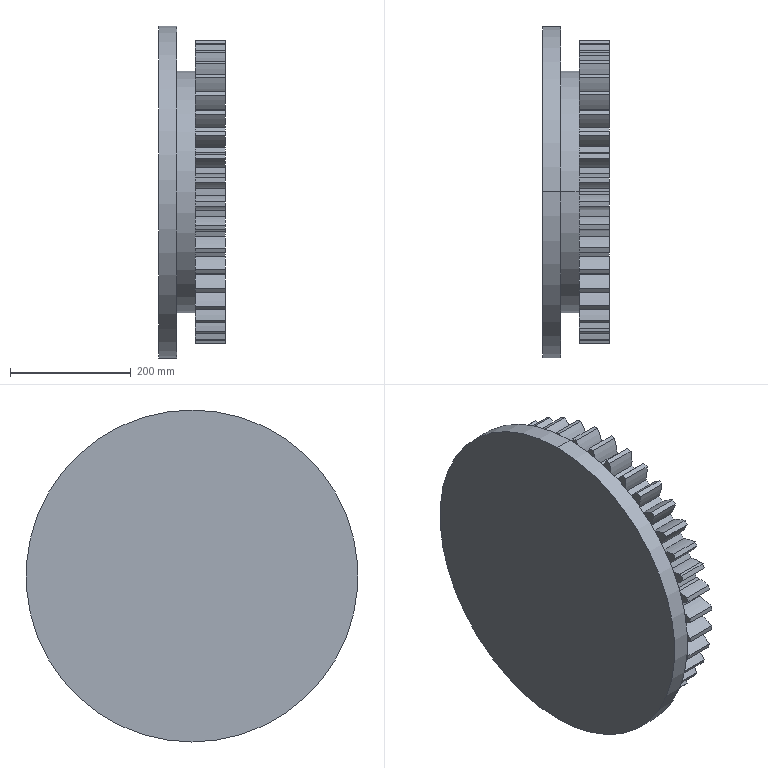Part | SolidWorks | features BaseBody 1 | 1 solid | 176 faces | box 110 x 550 x 550 mm | volume 19716444 mm3 | cylinder 171 | plane 5 | commonest cylinder face diameters 192 x84 449.998 x41 504 x40 50 x2 400 x2 550 x2